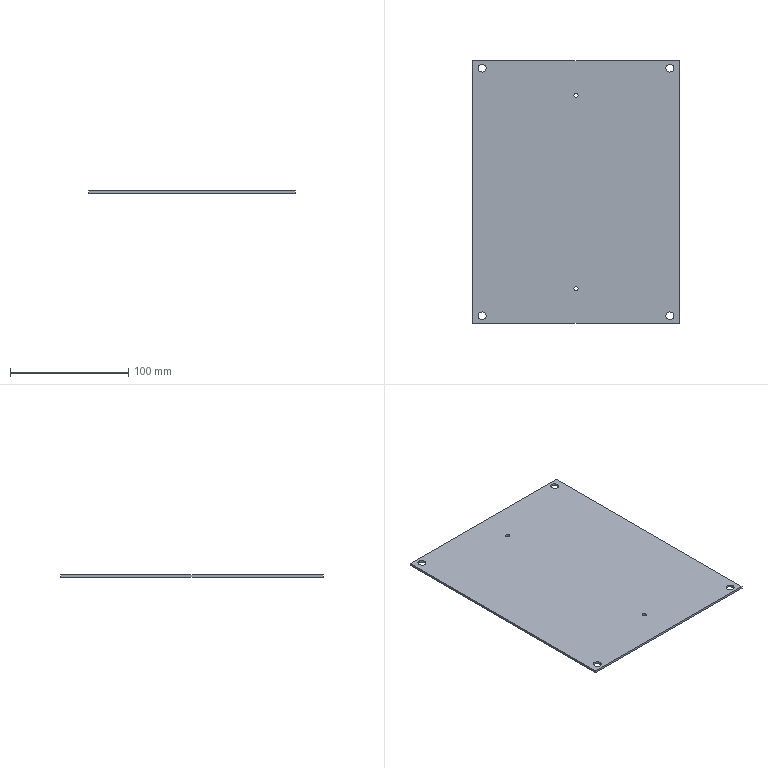Part | SolidWorks | features BaseBody 1 | 1 solid | 18 faces | box 174.625 x 222.25 x 1.829 mm | volume 70680 mm3 | cylinder 12 | plane 6 | commonest cylinder face diameters 6.731 x8 3.572 x4
STEP:
#1=CARTESIAN_POINT('',(79.375,108.141,-1.829));
#2=VERTEX_POINT('',#1);
#3=CARTESIAN_POINT('',(79.375,101.409,-1.829));
#4=VERTEX_POINT('',#3);
#5=CARTESIAN_POINT('',(79.375,104.775,-1.829));
#6=DIRECTION('',(0.,0.,1.));
#7=DIRECTION('',(0.,-1.,0.));
#8=AXIS2_PLACEMENT_3D('',#5,#6,#7);
#9=CIRCLE('',#8,3.365);
#10=EDGE_CURVE('',#2,#4,#9,.T.);
#11=ORIENTED_EDGE('',*,*,#10,.F.);
#12=CARTESIAN_POINT('',(79.375,108.141,0.));
#13=VERTEX_POINT('',#12);
#14=CARTESIAN_POINT('',(79.375,108.14,-282.652));
#15=DIRECTION('',(0.,0.,1.));
#16=VECTOR('',#15,1000.);
#17=LINE('',#14,#16);
#18=EDGE_CURVE('',#2,#13,#17,.T.);
#19=ORIENTED_EDGE('',*,*,#18,.T.);
#20=CARTESIAN_POINT('',(79.375,101.409,0.));
#21=VERTEX_POINT('',#20);
#22=CARTESIAN_POINT('',(79.375,104.775,0.));
#23=DIRECTION('',(0.,0.,1.));
#24=DIRECTION('',(1.,0.,0.));
#25=AXIS2_PLACEMENT_3D('',#22,#23,#24);
#26=CIRCLE('',#25,3.365);
#27=EDGE_CURVE('',#13,#21,#26,.T.);
#28=ORIENTED_EDGE('',*,*,#27,.T.);
#29=CARTESIAN_POINT('',(79.375,101.409,-282.652));
#30=DIRECTION('',(0.,0.,1.));
#31=VECTOR('',#30,1000.);
#32=LINE('',#29,#31);
#33=EDGE_CURVE('',#4,#21,#32,.T.);
#34=ORIENTED_EDGE('',*,*,#33,.F.);
#35=EDGE_LOOP('',(#11,#19,#28,#34));
#36=FACE_OUTER_BOUND('',#35,.T.);
#37=CARTESIAN_POINT('',(79.375,104.775,-282.652));
#38=DIRECTION('',(0.,0.,1.));
#39=DIRECTION('',(0.,-1.,0.));
#40=AXIS2_PLACEMENT_3D('',#37,#38,#39);
#41=CYLINDRICAL_SURFACE('',#40,3.365);
#42=ADVANCED_FACE('',(#36),#41,.F.);
#43=CARTESIAN_POINT('',(79.375,-101.409,-1.829));
#44=VERTEX_POINT('',#43);
#45=CARTESIAN_POINT('',(79.375,-108.14,-1.829));
#46=VERTEX_POINT('',#45);
#47=CARTESIAN_POINT('',(79.375,-104.775,-1.829));
#48=DIRECTION('',(0.,0.,1.));
#49=DIRECTION('',(0.,-1.,0.));
#50=AXIS2_PLACEMENT_3D('',#47,#48,#49);
#51=CIRCLE('',#50,3.365);
#52=EDGE_CURVE('',#44,#46,#51,.T.);
#53=ORIENTED_EDGE('',*,*,#52,.F.);
#54=CARTESIAN_POINT('',(79.375,-101.409,0.));
#55=VERTEX_POINT('',#54);
#56=CARTESIAN_POINT('',(79.375,-101.409,-282.652));
#57=DIRECTION('',(0.,0.,1.));
#58=VECTOR('',#57,1000.);
#59=LINE('',#56,#58);
#60=EDGE_CURVE('',#44,#55,#59,.T.);
#61=ORIENTED_EDGE('',*,*,#60,.T.);
#62=CARTESIAN_POINT('',(79.375,-108.141,0.));
#63=VERTEX_POINT('',#62);
#64=CARTESIAN_POINT('',(79.375,-104.775,0.));
#65=DIRECTION('',(0.,0.,1.));
#66=DIRECTION('',(1.,0.,0.));
#67=AXIS2_PLACEMENT_3D('',#64,#65,#66);
#68=CIRCLE('',#67,3.365);
#69=EDGE_CURVE('',#55,#63,#68,.T.);
#70=ORIENTED_EDGE('',*,*,#69,.T.);
#71=CARTESIAN_POINT('',(79.375,-108.14,-282.652));
#72=DIRECTION('',(0.,0.,1.));
#73=VECTOR('',#72,1000.);
#74=LINE('',#71,#73);
#75=EDGE_CURVE('',#46,#63,#74,.T.);
#76=ORIENTED_EDGE('',*,*,#75,.F.);
#77=EDGE_LOOP('',(#53,#61,#70,#76));
#78=FACE_OUTER_BOUND('',#77,.T.);
#79=CARTESIAN_POINT('',(79.375,-104.775,-282.652));
#80=DIRECTION('',(0.,0.,1.));
#81=DIRECTION('',(0.,-1.,0.));
#82=AXIS2_PLACEMENT_3D('',#79,#80,#81);
#83=CYLINDRICAL_SURFACE('',#82,3.365);
#84=ADVANCED_FACE('',(#78),#83,.F.);
#85=CARTESIAN_POINT('',(-79.375,108.141,-1.829));
#86=VERTEX_POINT('',#85);
#87=CARTESIAN_POINT('',(-79.375,101.409,-1.829));
#88=VERTEX_POINT('',#87);
#89=CARTESIAN_POINT('',(-79.375,104.775,-1.829));
#90=DIRECTION('',(0.,0.,1.));
#91=DIRECTION('',(0.,-1.,0.));
#92=AXIS2_PLACEMENT_3D('',#89,#90,#91);
#93=CIRCLE('',#92,3.365);
#94=EDGE_CURVE('',#86,#88,#93,.T.);
#95=ORIENTED_EDGE('',*,*,#94,.F.);
#96=CARTESIAN_POINT('',(-79.375,108.141,0.));
#97=VERTEX_POINT('',#96);
#98=CARTESIAN_POINT('',(-79.375,108.14,-282.652));
#99=DIRECTION('',(0.,0.,1.));
#100=VECTOR('',#99,1000.);
#101=LINE('',#98,#100);
#102=EDGE_CURVE('',#86,#97,#101,.T.);
#103=ORIENTED_EDGE('',*,*,#102,.T.);
#104=CARTESIAN_POINT('',(-79.375,101.409,0.));
#105=VERTEX_POINT('',#104);
#106=CARTESIAN_POINT('',(-79.375,104.775,0.));
#107=DIRECTION('',(0.,0.,1.));
#108=DIRECTION('',(1.,0.,0.));
#109=AXIS2_PLACEMENT_3D('',#106,#107,#108);
#110=CIRCLE('',#109,3.365);
#111=EDGE_CURVE('',#97,#105,#110,.T.);
#112=ORIENTED_EDGE('',*,*,#111,.T.);
#113=CARTESIAN_POINT('',(-79.375,101.409,-282.652));
#114=DIRECTION('',(0.,0.,1.));
#115=VECTOR('',#114,1000.);
#116=LINE('',#113,#115);
#117=EDGE_CURVE('',#88,#105,#116,.T.);
#118=ORIENTED_EDGE('',*,*,#117,.F.);
#119=EDGE_LOOP('',(#95,#103,#112,#118));
#120=FACE_OUTER_BOUND('',#119,.T.);
#121=CARTESIAN_POINT('',(-79.375,104.775,-282.652));
#122=DIRECTION('',(0.,0.,1.));
#123=DIRECTION('',(0.,-1.,0.));
#124=AXIS2_PLACEMENT_3D('',#121,#122,#123);
#125=CYLINDRICAL_SURFACE('',#124,3.365);
#126=ADVANCED_FACE('',(#120),#125,.F.);
#127=CARTESIAN_POINT('',(-79.375,-101.409,-1.829));
#128=VERTEX_POINT('',#127);
#129=CARTESIAN_POINT('',(-79.375,-108.14,-1.829));
#130=VERTEX_POINT('',#129);
#131=CARTESIAN_POINT('',(-79.375,-104.775,-1.829));
#132=DIRECTION('',(0.,0.,1.));
#133=DIRECTION('',(0.,-1.,0.));
#134=AXIS2_PLACEMENT_3D('',#131,#132,#133);
#135=CIRCLE('',#134,3.365);
#136=EDGE_CURVE('',#128,#130,#135,.T.);
#137=ORIENTED_EDGE('',*,*,#136,.F.);
#138=CARTESIAN_POINT('',(-79.375,-101.409,0.));
#139=VERTEX_POINT('',#138);
#140=CARTESIAN_POINT('',(-79.375,-101.409,-282.652));
#141=DIRECTION('',(0.,0.,1.));
#142=VECTOR('',#141,1000.);
#143=LINE('',#140,#142);
#144=EDGE_CURVE('',#128,#139,#143,.T.);
#145=ORIENTED_EDGE('',*,*,#144,.T.);
#146=CARTESIAN_POINT('',(-79.375,-108.141,0.));
#147=VERTEX_POINT('',#146);
#148=CARTESIAN_POINT('',(-79.375,-104.775,0.));
#149=DIRECTION('',(0.,0.,1.));
#150=DIRECTION('',(1.,0.,0.));
#151=AXIS2_PLACEMENT_3D('',#148,#149,#150);
#152=CIRCLE('',#151,3.365);
#153=EDGE_CURVE('',#139,#147,#152,.T.);
#154=ORIENTED_EDGE('',*,*,#153,.T.);
#155=CARTESIAN_POINT('',(-79.375,-108.14,-282.652));
#156=DIRECTION('',(0.,0.,1.));
#157=VECTOR('',#156,1000.);
#158=LINE('',#155,#157);
#159=EDGE_CURVE('',#130,#147,#158,.T.);
#160=ORIENTED_EDGE('',*,*,#159,.F.);
#161=EDGE_LOOP('',(#137,#145,#154,#160));
#162=FACE_OUTER_BOUND('',#161,.T.);
#163=CARTESIAN_POINT('',(-79.375,-104.775,-282.652));
#164=DIRECTION('',(0.,0.,1.));
#165=DIRECTION('',(0.,-1.,0.));
#166=AXIS2_PLACEMENT_3D('',#163,#164,#165);
#167=CYLINDRICAL_SURFACE('',#166,3.365);
#168=ADVANCED_FACE('',(#162),#167,.F.);
#169=CARTESIAN_POINT('',(0.,-83.436,-1.829));
#170=VERTEX_POINT('',#169);
#171=CARTESIAN_POINT('',(0.,-79.864,-1.829));
#172=VERTEX_POINT('',#171);
#173=CARTESIAN_POINT('',(0.,-81.65,-1.829));
#174=DIRECTION('',(0.,0.,-1.));
#175=DIRECTION('',(0.,-1.,0.));
#176=AXIS2_PLACEMENT_3D('',#173,#174,#175);
#177=CIRCLE('',#176,1.786);
#178=EDGE_CURVE('',#170,#172,#177,.T.);
#179=ORIENTED_EDGE('',*,*,#178,.T.);
#180=CARTESIAN_POINT('',(0.,-79.864,0.));
#181=VERTEX_POINT('',#180);
#182=CARTESIAN_POINT('',(0.,-79.864,-25.));
#183=DIRECTION('',(0.,0.,1.));
#184=VECTOR('',#183,1000.);
#185=LINE('',#182,#184);
#186=EDGE_CURVE('',#172,#181,#185,.T.);
#187=ORIENTED_EDGE('',*,*,#186,.T.);
#188=CARTESIAN_POINT('',(0.,-83.436,0.));
#189=VERTEX_POINT('',#188);
#190=CARTESIAN_POINT('',(0.,-81.65,0.));
#191=DIRECTION('',(0.,0.,-1.));
#192=DIRECTION('',(0.,-1.,0.));
#193=AXIS2_PLACEMENT_3D('',#190,#191,#192);
#194=CIRCLE('',#193,1.786);
#195=EDGE_CURVE('',#189,#181,#194,.T.);
#196=ORIENTED_EDGE('',*,*,#195,.F.);
#197=CARTESIAN_POINT('',(0.,-83.436,-25.));
#198=DIRECTION('',(0.,0.,1.));
#199=VECTOR('',#198,1000.);
#200=LINE('',#197,#199);
#201=EDGE_CURVE('',#170,#189,#200,.T.);
#202=ORIENTED_EDGE('',*,*,#201,.F.);
#203=EDGE_LOOP('',(#179,#187,#196,#202));
#204=FACE_OUTER_BOUND('',#203,.T.);
#205=CARTESIAN_POINT('',(0.,-81.65,-25.));
#206=DIRECTION('',(0.,0.,1.));
#207=DIRECTION('',(0.,-1.,0.));
#208=AXIS2_PLACEMENT_3D('',#205,#206,#207);
#209=CYLINDRICAL_SURFACE('',#208,1.786);
#210=ADVANCED_FACE('',(#204),#209,.F.);
#211=CARTESIAN_POINT('',(0.,83.436,-1.829));
#212=VERTEX_POINT('',#211);
#213=CARTESIAN_POINT('',(0.,79.864,-1.829));
#214=VERTEX_POINT('',#213);
#215=CARTESIAN_POINT('',(0.,81.65,-1.829));
#216=DIRECTION('',(0.,0.,1.));
#217=DIRECTION('',(0.,-1.,0.));
#218=AXIS2_PLACEMENT_3D('',#215,#216,#217);
#219=CIRCLE('',#218,1.786);
#220=EDGE_CURVE('',#212,#214,#219,.T.);
#221=ORIENTED_EDGE('',*,*,#220,.F.);
#222=CARTESIAN_POINT('',(0.,83.436,0.));
#223=VERTEX_POINT('',#222);
#224=CARTESIAN_POINT('',(0.,83.436,-25.));
#225=DIRECTION('',(0.,0.,1.));
#226=VECTOR('',#225,1000.);
#227=LINE('',#224,#226);
#228=EDGE_CURVE('',#212,#223,#227,.T.);
#229=ORIENTED_EDGE('',*,*,#228,.T.);
#230=CARTESIAN_POINT('',(0.,79.864,0.));
#231=VERTEX_POINT('',#230);
#232=CARTESIAN_POINT('',(0.,81.65,0.));
#233=DIRECTION('',(0.,0.,1.));
#234=DIRECTION('',(0.,-1.,0.));
#235=AXIS2_PLACEMENT_3D('',#232,#233,#234);
#236=CIRCLE('',#235,1.786);
#237=EDGE_CURVE('',#223,#231,#236,.T.);
#238=ORIENTED_EDGE('',*,*,#237,.T.);
#239=CARTESIAN_POINT('',(0.,79.864,-25.));
#240=DIRECTION('',(0.,0.,1.));
#241=VECTOR('',#240,1000.);
#242=LINE('',#239,#241);
#243=EDGE_CURVE('',#214,#231,#242,.T.);
#244=ORIENTED_EDGE('',*,*,#243,.F.);
#245=EDGE_LOOP('',(#221,#229,#238,#244));
#246=FACE_OUTER_BOUND('',#245,.T.);
#247=CARTESIAN_POINT('',(0.,81.65,-25.));
#248=DIRECTION('',(0.,0.,1.));
#249=DIRECTION('',(0.,-1.,0.));
#250=AXIS2_PLACEMENT_3D('',#247,#248,#249);
#251=CYLINDRICAL_SURFACE('',#250,1.786);
#252=ADVANCED_FACE('',(#246),#251,.F.);
#253=ORIENTED_EDGE('',*,*,#228,.F.);
#254=CARTESIAN_POINT('',(0.,81.65,-1.829));
#255=DIRECTION('',(0.,0.,1.));
#256=DIRECTION('',(0.,-1.,0.));
#257=AXIS2_PLACEMENT_3D('',#254,#255,#256);
#258=CIRCLE('',#257,1.786);
#259=EDGE_CURVE('',#214,#212,#258,.T.);
#260=ORIENTED_EDGE('',*,*,#259,.F.);
#261=ORIENTED_EDGE('',*,*,#243,.T.);
#262=CARTESIAN_POINT('',(0.,81.65,0.));
#263=DIRECTION('',(0.,0.,1.));
#264=DIRECTION('',(0.,-1.,0.));
#265=AXIS2_PLACEMENT_3D('',#262,#263,#264);
#266=CIRCLE('',#265,1.786);
#267=EDGE_CURVE('',#231,#223,#266,.T.);
#268=ORIENTED_EDGE('',*,*,#267,.T.);
#269=EDGE_LOOP('',(#253,#260,#261,#268));
#270=FACE_OUTER_BOUND('',#269,.T.);
#271=CARTESIAN_POINT('',(0.,81.65,-25.));
#272=DIRECTION('',(0.,0.,1.));
#273=DIRECTION('',(0.,-1.,0.));
#274=AXIS2_PLACEMENT_3D('',#271,#272,#273);
#275=CYLINDRICAL_SURFACE('',#274,1.786);
#276=ADVANCED_FACE('',(#270),#275,.F.);
#277=ORIENTED_EDGE('',*,*,#186,.F.);
#278=CARTESIAN_POINT('',(0.,-81.65,-1.829));
#279=DIRECTION('',(0.,0.,-1.));
#280=DIRECTION('',(0.,-1.,0.));
#281=AXIS2_PLACEMENT_3D('',#278,#279,#280);
#282=CIRCLE('',#281,1.786);
#283=EDGE_CURVE('',#172,#170,#282,.T.);
#284=ORIENTED_EDGE('',*,*,#283,.T.);
#285=ORIENTED_EDGE('',*,*,#201,.T.);
#286=CARTESIAN_POINT('',(0.,-81.65,0.));
#287=DIRECTION('',(0.,0.,-1.));
#288=DIRECTION('',(0.,-1.,0.));
#289=AXIS2_PLACEMENT_3D('',#286,#287,#288);
#290=CIRCLE('',#289,1.786);
#291=EDGE_CURVE('',#181,#189,#290,.T.);
#292=ORIENTED_EDGE('',*,*,#291,.F.);
#293=EDGE_LOOP('',(#277,#284,#285,#292));
#294=FACE_OUTER_BOUND('',#293,.T.);
#295=CARTESIAN_POINT('',(0.,-81.65,-25.));
#296=DIRECTION('',(0.,0.,1.));
#297=DIRECTION('',(0.,-1.,0.));
#298=AXIS2_PLACEMENT_3D('',#295,#296,#297);
#299=CYLINDRICAL_SURFACE('',#298,1.786);
#300=ADVANCED_FACE('',(#294),#299,.F.);
#301=CARTESIAN_POINT('',(-87.312,111.125,0.));
#302=VERTEX_POINT('',#301);
#303=CARTESIAN_POINT('',(-87.312,-111.125,0.));
#304=VERTEX_POINT('',#303);
#305=CARTESIAN_POINT('',(-87.312,111.125,0.));
#306=DIRECTION('',(0.,-1.,0.));
#307=VECTOR('',#306,1000.);
#308=LINE('',#305,#307);
#309=EDGE_CURVE('',#302,#304,#308,.T.);
#310=ORIENTED_EDGE('',*,*,#309,.F.);
#311=CARTESIAN_POINT('',(-87.312,111.125,-1.829));
#312=VERTEX_POINT('',#311);
#313=CARTESIAN_POINT('',(-87.312,111.125,-1.829));
#314=DIRECTION('',(0.,0.,1.));
#315=VECTOR('',#314,1000.);
#316=LINE('',#313,#315);
#317=EDGE_CURVE('',#312,#302,#316,.T.);
#318=ORIENTED_EDGE('',*,*,#317,.F.);
#319=CARTESIAN_POINT('',(-87.312,-111.125,-1.829));
#320=VERTEX_POINT('',#319);
#321=CARTESIAN_POINT('',(-87.312,111.125,-1.829));
#322=DIRECTION('',(0.,-1.,0.));
#323=VECTOR('',#322,1000.);
#324=LINE('',#321,#323);
#325=EDGE_CURVE('',#312,#320,#324,.T.);
#326=ORIENTED_EDGE('',*,*,#325,.T.);
#327=CARTESIAN_POINT('',(-87.312,-111.125,-1.829));
#328=DIRECTION('',(0.,0.,1.));
#329=VECTOR('',#328,1000.);
#330=LINE('',#327,#329);
#331=EDGE_CURVE('',#320,#304,#330,.T.);
#332=ORIENTED_EDGE('',*,*,#331,.T.);
#333=EDGE_LOOP('',(#310,#318,#326,#332));
#334=FACE_OUTER_BOUND('',#333,.T.);
#335=CARTESIAN_POINT('',(-87.312,111.125,-1.829));
#336=DIRECTION('',(-1.,0.,0.));
#337=DIRECTION('',(0.,0.,1.));
#338=AXIS2_PLACEMENT_3D('',#335,#336,#337);
#339=PLANE('',#338);
#340=ADVANCED_FACE('',(#334),#339,.T.);
#341=CARTESIAN_POINT('',(87.312,-111.125,0.));
#342=VERTEX_POINT('',#341);
#343=CARTESIAN_POINT('',(-87.312,-111.125,0.));
#344=DIRECTION('',(1.,0.,0.));
#345=VECTOR('',#344,1000.);
#346=LINE('',#343,#345);
#347=EDGE_CURVE('',#304,#342,#346,.T.);
#348=ORIENTED_EDGE('',*,*,#347,.F.);
#349=ORIENTED_EDGE('',*,*,#331,.F.);
#350=CARTESIAN_POINT('',(87.312,-111.125,-1.829));
#351=VERTEX_POINT('',#350);
#352=CARTESIAN_POINT('',(-87.312,-111.125,-1.829));
#353=DIRECTION('',(1.,0.,0.));
#354=VECTOR('',#353,1000.);
#355=LINE('',#352,#354);
#356=EDGE_CURVE('',#320,#351,#355,.T.);
#357=ORIENTED_EDGE('',*,*,#356,.T.);
#358=CARTESIAN_POINT('',(87.312,-111.125,-1.829));
#359=DIRECTION('',(0.,0.,1.));
#360=VECTOR('',#359,1000.);
#361=LINE('',#358,#360);
#362=EDGE_CURVE('',#351,#342,#361,.T.);
#363=ORIENTED_EDGE('',*,*,#362,.T.);
#364=EDGE_LOOP('',(#348,#349,#357,#363));
#365=FACE_OUTER_BOUND('',#364,.T.);
#366=CARTESIAN_POINT('',(-87.312,-111.125,-1.829));
#367=DIRECTION('',(0.,-1.,0.));
#368=DIRECTION('',(-1.,0.,0.));
#369=AXIS2_PLACEMENT_3D('',#366,#367,#368);
#370=PLANE('',#369);
#371=ADVANCED_FACE('',(#365),#370,.T.);
#372=CARTESIAN_POINT('',(87.312,111.125,0.));
#373=VERTEX_POINT('',#372);
#374=CARTESIAN_POINT('',(87.312,-111.125,0.));
#375=DIRECTION('',(0.,1.,0.));
#376=VECTOR('',#375,1000.);
#377=LINE('',#374,#376);
#378=EDGE_CURVE('',#342,#373,#377,.T.);
#379=ORIENTED_EDGE('',*,*,#378,.F.);
#380=ORIENTED_EDGE('',*,*,#362,.F.);
#381=CARTESIAN_POINT('',(87.312,111.125,-1.829));
#382=VERTEX_POINT('',#381);
#383=CARTESIAN_POINT('',(87.312,-111.125,-1.829));
#384=DIRECTION('',(0.,1.,0.));
#385=VECTOR('',#384,1000.);
#386=LINE('',#383,#385);
#387=EDGE_CURVE('',#351,#382,#386,.T.);
#388=ORIENTED_EDGE('',*,*,#387,.T.);
#389=CARTESIAN_POINT('',(87.312,111.125,-1.829));
#390=DIRECTION('',(0.,0.,1.));
#391=VECTOR('',#390,1000.);
#392=LINE('',#389,#391);
#393=EDGE_CURVE('',#382,#373,#392,.T.);
#394=ORIENTED_EDGE('',*,*,#393,.T.);
#395=EDGE_LOOP('',(#379,#380,#388,#394));
#396=FACE_OUTER_BOUND('',#395,.T.);
#397=CARTESIAN_POINT('',(87.312,-111.125,-1.829));
#398=DIRECTION('',(1.,0.,0.));
#399=DIRECTION('',(0.,1.,0.));
#400=AXIS2_PLACEMENT_3D('',#397,#398,#399);
#401=PLANE('',#400);
#402=ADVANCED_FACE('',(#396),#401,.T.);
#403=CARTESIAN_POINT('',(87.312,111.125,0.));
#404=DIRECTION('',(-1.,0.,0.));
#405=VECTOR('',#404,1000.);
#406=LINE('',#403,#405);
#407=EDGE_CURVE('',#373,#302,#406,.T.);
#408=ORIENTED_EDGE('',*,*,#407,.F.);
#409=ORIENTED_EDGE('',*,*,#393,.F.);
#410=CARTESIAN_POINT('',(87.312,111.125,-1.829));
#411=DIRECTION('',(-1.,0.,0.));
#412=VECTOR('',#411,1000.);
#413=LINE('',#410,#412);
#414=EDGE_CURVE('',#382,#312,#413,.T.);
#415=ORIENTED_EDGE('',*,*,#414,.T.);
#416=ORIENTED_EDGE('',*,*,#317,.T.);
#417=EDGE_LOOP('',(#408,#409,#415,#416));
#418=FACE_OUTER_BOUND('',#417,.T.);
#419=CARTESIAN_POINT('',(87.312,111.125,-1.829));
#420=DIRECTION('',(0.,1.,0.));
#421=DIRECTION('',(1.,0.,0.));
#422=AXIS2_PLACEMENT_3D('',#419,#420,#421);
#423=PLANE('',#422);
#424=ADVANCED_FACE('',(#418),#423,.T.);
#425=ORIENTED_EDGE('',*,*,#144,.F.);
#426=CARTESIAN_POINT('',(-79.375,-104.775,-1.829));
#427=DIRECTION('',(0.,0.,1.));
#428=DIRECTION('',(0.,-1.,0.));
#429=AXIS2_PLACEMENT_3D('',#426,#427,#428);
#430=CIRCLE('',#429,3.365);
#431=EDGE_CURVE('',#130,#128,#430,.T.);
#432=ORIENTED_EDGE('',*,*,#431,.F.);
#433=ORIENTED_EDGE('',*,*,#159,.T.);
#434=CARTESIAN_POINT('',(-79.375,-104.775,0.));
#435=DIRECTION('',(0.,0.,1.));
#436=DIRECTION('',(1.,0.,0.));
#437=AXIS2_PLACEMENT_3D('',#434,#435,#436);
#438=CIRCLE('',#437,3.365);
#439=EDGE_CURVE('',#147,#139,#438,.T.);
#440=ORIENTED_EDGE('',*,*,#439,.T.);
#441=EDGE_LOOP('',(#425,#432,#433,#440));
#442=FACE_OUTER_BOUND('',#441,.T.);
#443=CARTESIAN_POINT('',(-79.375,-104.775,-282.652));
#444=DIRECTION('',(0.,0.,1.));
#445=DIRECTION('',(0.,-1.,0.));
#446=AXIS2_PLACEMENT_3D('',#443,#444,#445);
#447=CYLINDRICAL_SURFACE('',#446,3.365);
#448=ADVANCED_FACE('',(#442),#447,.F.);
#449=ORIENTED_EDGE('',*,*,#102,.F.);
#450=CARTESIAN_POINT('',(-79.375,104.775,-1.829));
#451=DIRECTION('',(0.,0.,1.));
#452=DIRECTION('',(0.,-1.,0.));
#453=AXIS2_PLACEMENT_3D('',#450,#451,#452);
#454=CIRCLE('',#453,3.365);
#455=EDGE_CURVE('',#88,#86,#454,.T.);
#456=ORIENTED_EDGE('',*,*,#455,.F.);
#457=ORIENTED_EDGE('',*,*,#117,.T.);
#458=CARTESIAN_POINT('',(-79.375,104.775,0.));
#459=DIRECTION('',(0.,0.,1.));
#460=DIRECTION('',(1.,0.,0.));
#461=AXIS2_PLACEMENT_3D('',#458,#459,#460);
#462=CIRCLE('',#461,3.365);
#463=EDGE_CURVE('',#105,#97,#462,.T.);
#464=ORIENTED_EDGE('',*,*,#463,.T.);
#465=EDGE_LOOP('',(#449,#456,#457,#464));
#466=FACE_OUTER_BOUND('',#465,.T.);
#467=CARTESIAN_POINT('',(-79.375,104.775,-282.652));
#468=DIRECTION('',(0.,0.,1.));
#469=DIRECTION('',(0.,-1.,0.));
#470=AXIS2_PLACEMENT_3D('',#467,#468,#469);
#471=CYLINDRICAL_SURFACE('',#470,3.365);
#472=ADVANCED_FACE('',(#466),#471,.F.);
#473=ORIENTED_EDGE('',*,*,#60,.F.);
#474=CARTESIAN_POINT('',(79.375,-104.775,-1.829));
#475=DIRECTION('',(0.,0.,1.));
#476=DIRECTION('',(0.,-1.,0.));
#477=AXIS2_PLACEMENT_3D('',#474,#475,#476);
#478=CIRCLE('',#477,3.365);
#479=EDGE_CURVE('',#46,#44,#478,.T.);
#480=ORIENTED_EDGE('',*,*,#479,.F.);
#481=ORIENTED_EDGE('',*,*,#75,.T.);
#482=CARTESIAN_POINT('',(79.375,-104.775,0.));
#483=DIRECTION('',(0.,0.,1.));
#484=DIRECTION('',(1.,0.,0.));
#485=AXIS2_PLACEMENT_3D('',#482,#483,#484);
#486=CIRCLE('',#485,3.365);
#487=EDGE_CURVE('',#63,#55,#486,.T.);
#488=ORIENTED_EDGE('',*,*,#487,.T.);
#489=EDGE_LOOP('',(#473,#480,#481,#488));
#490=FACE_OUTER_BOUND('',#489,.T.);
#491=CARTESIAN_POINT('',(79.375,-104.775,-282.652));
#492=DIRECTION('',(0.,0.,1.));
#493=DIRECTION('',(0.,-1.,0.));
#494=AXIS2_PLACEMENT_3D('',#491,#492,#493);
#495=CYLINDRICAL_SURFACE('',#494,3.365);
#496=ADVANCED_FACE('',(#490),#495,.F.);
#497=ORIENTED_EDGE('',*,*,#18,.F.);
#498=CARTESIAN_POINT('',(79.375,104.775,-1.829));
#499=DIRECTION('',(0.,0.,1.));
#500=DIRECTION('',(0.,-1.,0.));
#501=AXIS2_PLACEMENT_3D('',#498,#499,#500);
#502=CIRCLE('',#501,3.365);
#503=EDGE_CURVE('',#4,#2,#502,.T.);
#504=ORIENTED_EDGE('',*,*,#503,.F.);
#505=ORIENTED_EDGE('',*,*,#33,.T.);
#506=CARTESIAN_POINT('',(79.375,104.775,0.));
#507=DIRECTION('',(0.,0.,1.));
#508=DIRECTION('',(1.,0.,0.));
#509=AXIS2_PLACEMENT_3D('',#506,#507,#508);
#510=CIRCLE('',#509,3.365);
#511=EDGE_CURVE('',#21,#13,#510,.T.);
#512=ORIENTED_EDGE('',*,*,#511,.T.);
#513=EDGE_LOOP('',(#497,#504,#505,#512));
#514=FACE_OUTER_BOUND('',#513,.T.);
#515=CARTESIAN_POINT('',(79.375,104.775,-282.652));
#516=DIRECTION('',(0.,0.,1.));
#517=DIRECTION('',(0.,-1.,0.));
#518=AXIS2_PLACEMENT_3D('',#515,#516,#517);
#519=CYLINDRICAL_SURFACE('',#518,3.365);
#520=ADVANCED_FACE('',(#514),#519,.F.);
#521=ORIENTED_EDGE('',*,*,#259,.T.);
#522=ORIENTED_EDGE('',*,*,#220,.T.);
#523=EDGE_LOOP('',(#521,#522));
#524=FACE_BOUND('',#523,.T.);
#525=ORIENTED_EDGE('',*,*,#178,.F.);
#526=ORIENTED_EDGE('',*,*,#283,.F.);
#527=EDGE_LOOP('',(#525,#526));
#528=FACE_BOUND('',#527,.T.);
#529=ORIENTED_EDGE('',*,*,#325,.F.);
#530=ORIENTED_EDGE('',*,*,#414,.F.);
#531=ORIENTED_EDGE('',*,*,#387,.F.);
#532=ORIENTED_EDGE('',*,*,#356,.F.);
#533=EDGE_LOOP('',(#529,#530,#531,#532));
#534=FACE_OUTER_BOUND('',#533,.T.);
#535=ORIENTED_EDGE('',*,*,#431,.T.);
#536=ORIENTED_EDGE('',*,*,#136,.T.);
#537=EDGE_LOOP('',(#535,#536));
#538=FACE_BOUND('',#537,.T.);
#539=ORIENTED_EDGE('',*,*,#455,.T.);
#540=ORIENTED_EDGE('',*,*,#94,.T.);
#541=EDGE_LOOP('',(#539,#540));
#542=FACE_BOUND('',#541,.T.);
#543=ORIENTED_EDGE('',*,*,#479,.T.);
#544=ORIENTED_EDGE('',*,*,#52,.T.);
#545=EDGE_LOOP('',(#543,#544));
#546=FACE_BOUND('',#545,.T.);
#547=ORIENTED_EDGE('',*,*,#503,.T.);
#548=ORIENTED_EDGE('',*,*,#10,.T.);
#549=EDGE_LOOP('',(#547,#548));
#550=FACE_BOUND('',#549,.T.);
#551=CARTESIAN_POINT('',(-87.312,-111.125,-1.829));
#552=DIRECTION('',(0.,0.,1.));
#553=DIRECTION('',(1.,0.,0.));
#554=AXIS2_PLACEMENT_3D('',#551,#552,#553);
#555=PLANE('',#554);
#556=ADVANCED_FACE('',(#524,#528,#534,#538,#542,#546,#550),#555,.F.);
#557=ORIENTED_EDGE('',*,*,#267,.F.);
#558=ORIENTED_EDGE('',*,*,#237,.F.);
#559=EDGE_LOOP('',(#557,#558));
#560=FACE_BOUND('',#559,.T.);
#561=ORIENTED_EDGE('',*,*,#511,.F.);
#562=ORIENTED_EDGE('',*,*,#27,.F.);
#563=EDGE_LOOP('',(#561,#562));
#564=FACE_BOUND('',#563,.T.);
#565=ORIENTED_EDGE('',*,*,#487,.F.);
#566=ORIENTED_EDGE('',*,*,#69,.F.);
#567=EDGE_LOOP('',(#565,#566));
#568=FACE_BOUND('',#567,.T.);
#569=ORIENTED_EDGE('',*,*,#463,.F.);
#570=ORIENTED_EDGE('',*,*,#111,.F.);
#571=EDGE_LOOP('',(#569,#570));
#572=FACE_BOUND('',#571,.T.);
#573=ORIENTED_EDGE('',*,*,#439,.F.);
#574=ORIENTED_EDGE('',*,*,#153,.F.);
#575=EDGE_LOOP('',(#573,#574));
#576=FACE_BOUND('',#575,.T.);
#577=ORIENTED_EDGE('',*,*,#309,.T.);
#578=ORIENTED_EDGE('',*,*,#347,.T.);
#579=ORIENTED_EDGE('',*,*,#378,.T.);
#580=ORIENTED_EDGE('',*,*,#407,.T.);
#581=EDGE_LOOP('',(#577,#578,#579,#580));
#582=FACE_OUTER_BOUND('',#581,.T.);
#583=ORIENTED_EDGE('',*,*,#195,.T.);
#584=ORIENTED_EDGE('',*,*,#291,.T.);
#585=EDGE_LOOP('',(#583,#584));
#586=FACE_BOUND('',#585,.T.);
#587=CARTESIAN_POINT('',(-87.312,-111.125,0.));
#588=DIRECTION('',(0.,0.,1.));
#589=DIRECTION('',(1.,0.,0.));
#590=AXIS2_PLACEMENT_3D('',#587,#588,#589);
#591=PLANE('',#590);
#592=ADVANCED_FACE('',(#560,#564,#568,#572,#576,#582,#586),#591,.T.);
#593=CLOSED_SHELL('',(#42,#84,#126,#168,#210,#252,#276,#300,#340,#371,#402,#424,#448,#472,#496,#520,#556,#592));
#594=MANIFOLD_SOLID_BREP('',#593);
#595=CARTESIAN_POINT('',(0.,0.,0.));
#596=DIRECTION('',(0.,0.,1.));
#597=DIRECTION('',(1.,0.,0.));
#598=AXIS2_PLACEMENT_3D('',#595,#596,#597);
#599=(LENGTH_UNIT()NAMED_UNIT(*)SI_UNIT(.MILLI.,.METRE.));
#600=UNCERTAINTY_MEASURE_WITH_UNIT(LENGTH_MEASURE(0.00001),#599,'','');
#601=(NAMED_UNIT(*)PLANE_ANGLE_UNIT()SI_UNIT($,.RADIAN.));
#602=(NAMED_UNIT(*)SI_UNIT($,.STERADIAN.)SOLID_ANGLE_UNIT());
#603=(GEOMETRIC_REPRESENTATION_CONTEXT(3)GLOBAL_UNCERTAINTY_ASSIGNED_CONTEXT((#600))GLOBAL_UNIT_ASSIGNED_CONTEXT((#599,#601,#602))REPRESENTATION_CONTEXT('',''));
#604=ADVANCED_BREP_SHAPE_REPRESENTATION('',(#594,#598),#603);